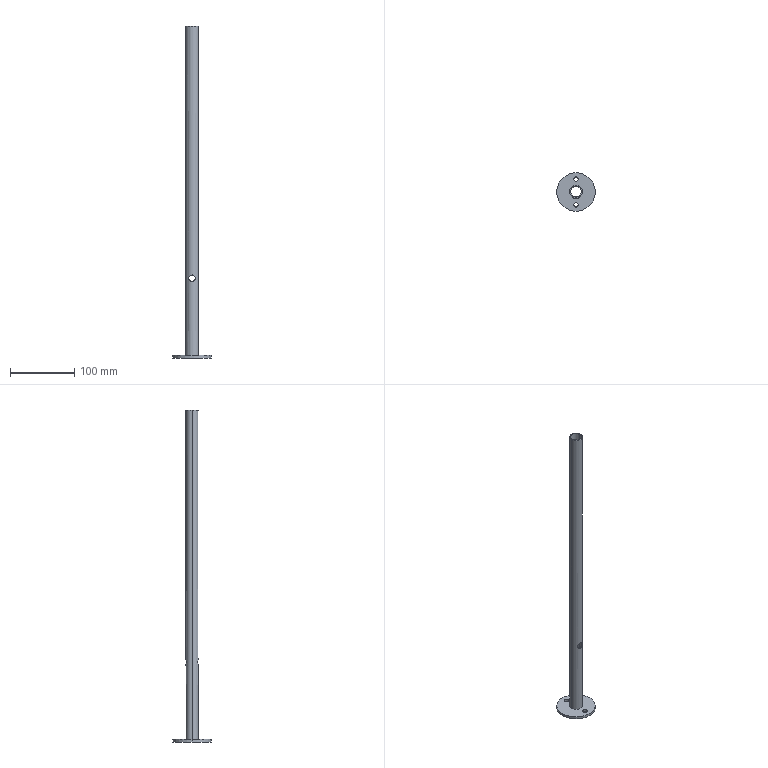Part | STEP file | Switch support rod 1_default<machined> | 2 solids | 24 faces | box 60 x 60 x 516 mm | volume 54480 mm3 | cylinder 16 | plane 4 | cone 4 | commonest cylinder face diameters 7 x4 10 x4 20 x4 17 x2 60 x2